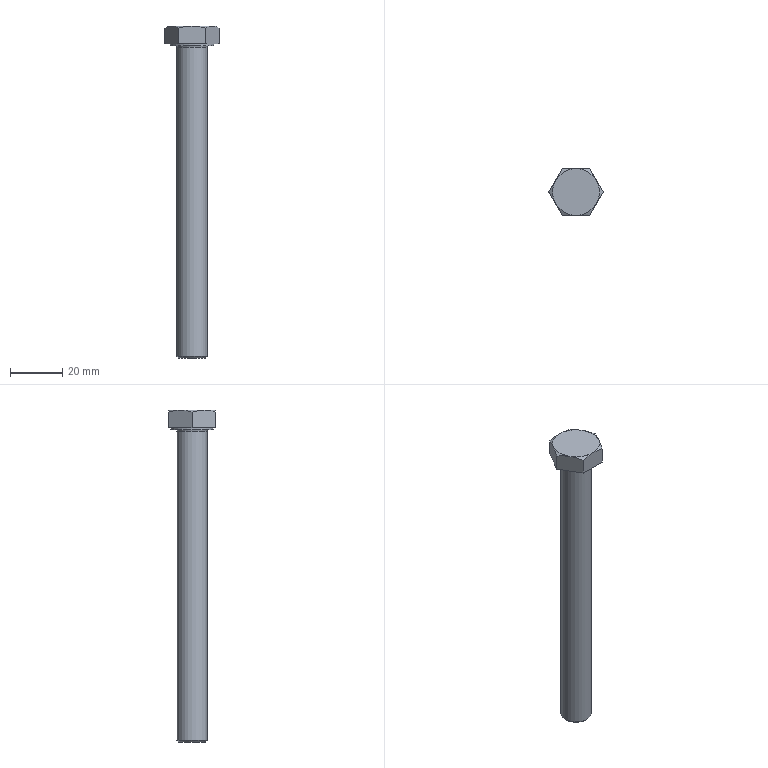Part | NX | features SKETCH 4, EXTRUDE 3, META 3, DATUM_CSYS 2, BLEND 1, CHAMFER 1, LINE 1, SWP104 1, SYMBOLIC_THREAD 1, THREADS 1 | 1 solid | 20 faces | box 20.785 x 18 x 127.5 mm | volume 14961 mm3 | plane 10 | cone 7 | cylinder 2 | torus 1 | commonest cylinder face diameters 11.701 x1 16.63 x1
STEP:
#1=CARTESIAN_POINT('',(5.196,-9.,0.6));
#2=VERTEX_POINT('',#1);
#3=CARTESIAN_POINT('',(10.392,0.,0.6));
#4=VERTEX_POINT('',#3);
#5=CARTESIAN_POINT('',(5.196,-9.,0.6));
#6=DIRECTION('',(0.5,0.866,0.));
#7=VECTOR('',#6,1000.);
#8=LINE('',#5,#7);
#9=EDGE_CURVE('',#2,#4,#8,.T.);
#10=ORIENTED_EDGE('',*,*,#9,.F.);
#11=CARTESIAN_POINT('',(-5.196,-9.,0.6));
#12=VERTEX_POINT('',#11);
#13=CARTESIAN_POINT('',(-5.196,-9.,0.6));
#14=DIRECTION('',(1.,0.,0.));
#15=VECTOR('',#14,1000.);
#16=LINE('',#13,#15);
#17=EDGE_CURVE('',#12,#2,#16,.T.);
#18=ORIENTED_EDGE('',*,*,#17,.F.);
#19=CARTESIAN_POINT('',(-10.392,0.,0.6));
#20=VERTEX_POINT('',#19);
#21=CARTESIAN_POINT('',(-10.392,0.,0.6));
#22=DIRECTION('',(0.5,-0.866,0.));
#23=VECTOR('',#22,1000.);
#24=LINE('',#21,#23);
#25=EDGE_CURVE('',#20,#12,#24,.T.);
#26=ORIENTED_EDGE('',*,*,#25,.F.);
#27=CARTESIAN_POINT('',(-5.196,9.,0.6));
#28=VERTEX_POINT('',#27);
#29=CARTESIAN_POINT('',(-5.196,9.,0.6));
#30=DIRECTION('',(-0.5,-0.866,0.));
#31=VECTOR('',#30,1000.);
#32=LINE('',#29,#31);
#33=EDGE_CURVE('',#28,#20,#32,.T.);
#34=ORIENTED_EDGE('',*,*,#33,.F.);
#35=CARTESIAN_POINT('',(5.196,9.,0.6));
#36=VERTEX_POINT('',#35);
#37=CARTESIAN_POINT('',(5.196,9.,0.6));
#38=DIRECTION('',(-1.,0.,0.));
#39=VECTOR('',#38,1000.);
#40=LINE('',#37,#39);
#41=EDGE_CURVE('',#36,#28,#40,.T.);
#42=ORIENTED_EDGE('',*,*,#41,.F.);
#43=CARTESIAN_POINT('',(10.392,0.,0.6));
#44=DIRECTION('',(-0.5,0.866,0.));
#45=VECTOR('',#44,1000.);
#46=LINE('',#43,#45);
#47=EDGE_CURVE('',#4,#36,#46,.T.);
#48=ORIENTED_EDGE('',*,*,#47,.F.);
#49=EDGE_LOOP('',(#10,#18,#26,#34,#42,#48));
#50=FACE_BOUND('',#49,.T.);
#51=CARTESIAN_POINT('',(8.315,0.,0.6));
#52=VERTEX_POINT('',#51);
#53=CARTESIAN_POINT('',(0.,0.,0.6));
#54=DIRECTION('',(0.,0.,1.));
#55=DIRECTION('',(1.,0.,0.));
#56=AXIS2_PLACEMENT_3D('',#53,#54,#55);
#57=CIRCLE('',#56,8.315);
#58=EDGE_CURVE('',#52,#52,#57,.T.);
#59=ORIENTED_EDGE('',*,*,#58,.T.);
#60=EDGE_LOOP('',(#59));
#61=FACE_BOUND('',#60,.T.);
#62=CARTESIAN_POINT('',(0.,-18.,0.6));
#63=DIRECTION('',(0.,0.,-1.));
#64=DIRECTION('',(-1.,0.,0.));
#65=AXIS2_PLACEMENT_3D('',#62,#63,#64);
#66=PLANE('',#65);
#67=ADVANCED_FACE('',(#50,#61),#66,.T.);
#68=CARTESIAN_POINT('',(5.196,-9.,6.696));
#69=VERTEX_POINT('',#68);
#70=CARTESIAN_POINT('',(7.794,-4.5,7.5));
#71=VERTEX_POINT('',#70);
#72=CARTESIAN_POINT('',(5.196,-9.,6.696));
#73=CARTESIAN_POINT('',(6.046,-7.528,7.187));
#74=CARTESIAN_POINT('',(6.909,-6.033,7.5));
#75=CARTESIAN_POINT('',(7.794,-4.5,7.5));
#76=B_SPLINE_CURVE_WITH_KNOTS('',3,(#72,#73,#74,#75),.UNSPECIFIED.,.F.,.F.,(4,4),(0.000000238,0.005258),.UNSPECIFIED.);
#77=EDGE_CURVE('',#69,#71,#76,.T.);
#78=ORIENTED_EDGE('',*,*,#77,.F.);
#79=CARTESIAN_POINT('',(5.196,-9.,7.5));
#80=DIRECTION('',(0.,0.,-1.));
#81=VECTOR('',#80,1000.);
#82=LINE('',#79,#81);
#83=EDGE_CURVE('',#69,#2,#82,.T.);
#84=ORIENTED_EDGE('',*,*,#83,.T.);
#85=ORIENTED_EDGE('',*,*,#9,.T.);
#86=CARTESIAN_POINT('',(10.392,0.,6.696));
#87=VERTEX_POINT('',#86);
#88=CARTESIAN_POINT('',(10.392,0.,7.5));
#89=DIRECTION('',(0.,0.,-1.));
#90=VECTOR('',#89,1000.);
#91=LINE('',#88,#90);
#92=EDGE_CURVE('',#87,#4,#91,.T.);
#93=ORIENTED_EDGE('',*,*,#92,.F.);
#94=CARTESIAN_POINT('',(7.794,-4.5,7.5));
#95=CARTESIAN_POINT('',(8.676,-2.972,7.5));
#96=CARTESIAN_POINT('',(9.544,-1.469,7.186));
#97=CARTESIAN_POINT('',(10.392,0.,6.696));
#98=B_SPLINE_CURVE_WITH_KNOTS('',3,(#94,#95,#96,#97),.UNSPECIFIED.,.F.,.F.,(4,4),(0.005258,0.0105),.UNSPECIFIED.);
#99=EDGE_CURVE('',#71,#87,#98,.T.);
#100=ORIENTED_EDGE('',*,*,#99,.F.);
#101=EDGE_LOOP('',(#78,#84,#85,#93,#100));
#102=FACE_BOUND('',#101,.T.);
#103=CARTESIAN_POINT('',(5.196,-9.,7.5));
#104=DIRECTION('',(-0.866,0.5,0.));
#105=DIRECTION('',(-0.5,-0.866,0.));
#106=AXIS2_PLACEMENT_3D('',#103,#104,#105);
#107=PLANE('',#106);
#108=ADVANCED_FACE('',(#102),#107,.F.);
#109=CARTESIAN_POINT('',(7.794,4.5,7.5));
#110=VERTEX_POINT('',#109);
#111=CARTESIAN_POINT('',(10.392,0.,6.696));
#112=CARTESIAN_POINT('',(9.542,1.472,7.187));
#113=CARTESIAN_POINT('',(8.679,2.967,7.5));
#114=CARTESIAN_POINT('',(7.794,4.5,7.5));
#115=B_SPLINE_CURVE_WITH_KNOTS('',3,(#111,#112,#113,#114),.UNSPECIFIED.,.F.,.F.,(4,4),(0.000000238,0.005258),.UNSPECIFIED.);
#116=EDGE_CURVE('',#87,#110,#115,.T.);
#117=ORIENTED_EDGE('',*,*,#116,.F.);
#118=ORIENTED_EDGE('',*,*,#92,.T.);
#119=ORIENTED_EDGE('',*,*,#47,.T.);
#120=CARTESIAN_POINT('',(5.196,9.,6.696));
#121=VERTEX_POINT('',#120);
#122=CARTESIAN_POINT('',(5.196,9.,7.5));
#123=DIRECTION('',(0.,0.,-1.));
#124=VECTOR('',#123,1000.);
#125=LINE('',#122,#124);
#126=EDGE_CURVE('',#121,#36,#125,.T.);
#127=ORIENTED_EDGE('',*,*,#126,.F.);
#128=CARTESIAN_POINT('',(7.794,4.5,7.5));
#129=CARTESIAN_POINT('',(6.912,6.028,7.5));
#130=CARTESIAN_POINT('',(6.044,7.531,7.186));
#131=CARTESIAN_POINT('',(5.196,9.,6.696));
#132=B_SPLINE_CURVE_WITH_KNOTS('',3,(#128,#129,#130,#131),.UNSPECIFIED.,.F.,.F.,(4,4),(0.005258,0.0105),.UNSPECIFIED.);
#133=EDGE_CURVE('',#110,#121,#132,.T.);
#134=ORIENTED_EDGE('',*,*,#133,.F.);
#135=EDGE_LOOP('',(#117,#118,#119,#127,#134));
#136=FACE_BOUND('',#135,.T.);
#137=CARTESIAN_POINT('',(10.392,0.,7.5));
#138=DIRECTION('',(-0.866,-0.5,0.));
#139=DIRECTION('',(0.5,-0.866,0.));
#140=AXIS2_PLACEMENT_3D('',#137,#138,#139);
#141=PLANE('',#140);
#142=ADVANCED_FACE('',(#136),#141,.F.);
#143=CARTESIAN_POINT('',(0.,9.,7.5));
#144=VERTEX_POINT('',#143);
#145=CARTESIAN_POINT('',(0.,9.,7.5));
#146=CARTESIAN_POINT('',(1.757,9.,7.5));
#147=CARTESIAN_POINT('',(3.516,9.,7.181));
#148=CARTESIAN_POINT('',(5.196,9.,6.696));
#149=B_SPLINE_CURVE_WITH_KNOTS('',3,(#145,#146,#147,#148),.UNSPECIFIED.,.F.,.F.,(4,4),(0.01453,0.01979),.UNSPECIFIED.);
#150=EDGE_CURVE('',#121,#144,#149,.F.);
#151=ORIENTED_EDGE('',*,*,#150,.F.);
#152=ORIENTED_EDGE('',*,*,#126,.T.);
#153=ORIENTED_EDGE('',*,*,#41,.T.);
#154=CARTESIAN_POINT('',(-5.196,9.,6.696));
#155=VERTEX_POINT('',#154);
#156=CARTESIAN_POINT('',(-5.196,9.,7.5));
#157=DIRECTION('',(0.,0.,-1.));
#158=VECTOR('',#157,1000.);
#159=LINE('',#156,#158);
#160=EDGE_CURVE('',#155,#28,#159,.T.);
#161=ORIENTED_EDGE('',*,*,#160,.F.);
#162=CARTESIAN_POINT('',(-5.196,9.,6.696));
#163=CARTESIAN_POINT('',(-3.506,9.,7.184));
#164=CARTESIAN_POINT('',(-1.756,9.,7.5));
#165=CARTESIAN_POINT('',(0.,9.,7.5));
#166=B_SPLINE_CURVE_WITH_KNOTS('',3,(#162,#163,#164,#165),.UNSPECIFIED.,.F.,.F.,(4,4),(0.009271,0.01453),.UNSPECIFIED.);
#167=EDGE_CURVE('',#144,#155,#166,.F.);
#168=ORIENTED_EDGE('',*,*,#167,.F.);
#169=EDGE_LOOP('',(#151,#152,#153,#161,#168));
#170=FACE_BOUND('',#169,.T.);
#171=CARTESIAN_POINT('',(5.196,9.,7.5));
#172=DIRECTION('',(0.,-1.,0.));
#173=DIRECTION('',(0.,0.,-1.));
#174=AXIS2_PLACEMENT_3D('',#171,#172,#173);
#175=PLANE('',#174);
#176=ADVANCED_FACE('',(#170),#175,.F.);
#177=CARTESIAN_POINT('',(-7.794,4.5,7.5));
#178=VERTEX_POINT('',#177);
#179=CARTESIAN_POINT('',(-5.196,9.,6.696));
#180=CARTESIAN_POINT('',(-6.046,7.528,7.187));
#181=CARTESIAN_POINT('',(-6.909,6.033,7.5));
#182=CARTESIAN_POINT('',(-7.794,4.5,7.5));
#183=B_SPLINE_CURVE_WITH_KNOTS('',3,(#179,#180,#181,#182),.UNSPECIFIED.,.F.,.F.,(4,4),(0.000000238,0.005258),.UNSPECIFIED.);
#184=EDGE_CURVE('',#155,#178,#183,.T.);
#185=ORIENTED_EDGE('',*,*,#184,.F.);
#186=ORIENTED_EDGE('',*,*,#160,.T.);
#187=ORIENTED_EDGE('',*,*,#33,.T.);
#188=CARTESIAN_POINT('',(-10.392,0.,6.696));
#189=VERTEX_POINT('',#188);
#190=CARTESIAN_POINT('',(-10.392,0.,7.5));
#191=DIRECTION('',(0.,0.,-1.));
#192=VECTOR('',#191,1000.);
#193=LINE('',#190,#192);
#194=EDGE_CURVE('',#189,#20,#193,.T.);
#195=ORIENTED_EDGE('',*,*,#194,.F.);
#196=CARTESIAN_POINT('',(-7.794,4.5,7.5));
#197=CARTESIAN_POINT('',(-8.676,2.972,7.5));
#198=CARTESIAN_POINT('',(-9.544,1.469,7.186));
#199=CARTESIAN_POINT('',(-10.392,0.,6.696));
#200=B_SPLINE_CURVE_WITH_KNOTS('',3,(#196,#197,#198,#199),.UNSPECIFIED.,.F.,.F.,(4,4),(0.005258,0.0105),.UNSPECIFIED.);
#201=EDGE_CURVE('',#178,#189,#200,.T.);
#202=ORIENTED_EDGE('',*,*,#201,.F.);
#203=EDGE_LOOP('',(#185,#186,#187,#195,#202));
#204=FACE_BOUND('',#203,.T.);
#205=CARTESIAN_POINT('',(-5.196,9.,7.5));
#206=DIRECTION('',(0.866,-0.5,0.));
#207=DIRECTION('',(0.5,0.866,0.));
#208=AXIS2_PLACEMENT_3D('',#205,#206,#207);
#209=PLANE('',#208);
#210=ADVANCED_FACE('',(#204),#209,.F.);
#211=CARTESIAN_POINT('',(-7.794,-4.5,7.5));
#212=VERTEX_POINT('',#211);
#213=CARTESIAN_POINT('',(-10.392,0.,6.696));
#214=CARTESIAN_POINT('',(-9.542,-1.472,7.187));
#215=CARTESIAN_POINT('',(-8.679,-2.967,7.5));
#216=CARTESIAN_POINT('',(-7.794,-4.5,7.5));
#217=B_SPLINE_CURVE_WITH_KNOTS('',3,(#213,#214,#215,#216),.UNSPECIFIED.,.F.,.F.,(4,4),(0.000000238,0.005258),.UNSPECIFIED.);
#218=EDGE_CURVE('',#189,#212,#217,.T.);
#219=ORIENTED_EDGE('',*,*,#218,.F.);
#220=ORIENTED_EDGE('',*,*,#194,.T.);
#221=ORIENTED_EDGE('',*,*,#25,.T.);
#222=CARTESIAN_POINT('',(-5.196,-9.,6.696));
#223=VERTEX_POINT('',#222);
#224=CARTESIAN_POINT('',(-5.196,-9.,7.5));
#225=DIRECTION('',(0.,0.,-1.));
#226=VECTOR('',#225,1000.);
#227=LINE('',#224,#226);
#228=EDGE_CURVE('',#223,#12,#227,.T.);
#229=ORIENTED_EDGE('',*,*,#228,.F.);
#230=CARTESIAN_POINT('',(-7.794,-4.5,7.5));
#231=CARTESIAN_POINT('',(-6.912,-6.028,7.5));
#232=CARTESIAN_POINT('',(-6.044,-7.531,7.186));
#233=CARTESIAN_POINT('',(-5.196,-9.,6.696));
#234=B_SPLINE_CURVE_WITH_KNOTS('',3,(#230,#231,#232,#233),.UNSPECIFIED.,.F.,.F.,(4,4),(0.005258,0.0105),.UNSPECIFIED.);
#235=EDGE_CURVE('',#212,#223,#234,.T.);
#236=ORIENTED_EDGE('',*,*,#235,.F.);
#237=EDGE_LOOP('',(#219,#220,#221,#229,#236));
#238=FACE_BOUND('',#237,.T.);
#239=CARTESIAN_POINT('',(-10.392,0.,7.5));
#240=DIRECTION('',(0.866,0.5,0.));
#241=DIRECTION('',(-0.5,0.866,0.));
#242=AXIS2_PLACEMENT_3D('',#239,#240,#241);
#243=PLANE('',#242);
#244=ADVANCED_FACE('',(#238),#243,.F.);
#245=CARTESIAN_POINT('',(0.,-9.,7.5));
#246=VERTEX_POINT('',#245);
#247=CARTESIAN_POINT('',(-5.196,-9.,6.696));
#248=CARTESIAN_POINT('',(-3.506,-9.,7.184));
#249=CARTESIAN_POINT('',(-1.756,-9.,7.5));
#250=CARTESIAN_POINT('',(0.,-9.,7.5));
#251=B_SPLINE_CURVE_WITH_KNOTS('',3,(#247,#248,#249,#250),.UNSPECIFIED.,.F.,.F.,(4,4),(0.009271,0.01453),.UNSPECIFIED.);
#252=EDGE_CURVE('',#223,#246,#251,.T.);
#253=ORIENTED_EDGE('',*,*,#252,.F.);
#254=ORIENTED_EDGE('',*,*,#228,.T.);
#255=ORIENTED_EDGE('',*,*,#17,.T.);
#256=ORIENTED_EDGE('',*,*,#83,.F.);
#257=CARTESIAN_POINT('',(0.,-9.,7.5));
#258=CARTESIAN_POINT('',(1.757,-9.,7.5));
#259=CARTESIAN_POINT('',(3.516,-9.,7.181));
#260=CARTESIAN_POINT('',(5.196,-9.,6.696));
#261=B_SPLINE_CURVE_WITH_KNOTS('',3,(#257,#258,#259,#260),.UNSPECIFIED.,.F.,.F.,(4,4),(0.01453,0.01979),.UNSPECIFIED.);
#262=EDGE_CURVE('',#246,#69,#261,.T.);
#263=ORIENTED_EDGE('',*,*,#262,.F.);
#264=EDGE_LOOP('',(#253,#254,#255,#256,#263));
#265=FACE_BOUND('',#264,.T.);
#266=CARTESIAN_POINT('',(-5.196,-9.,7.5));
#267=DIRECTION('',(0.,1.,0.));
#268=DIRECTION('',(0.,0.,1.));
#269=AXIS2_PLACEMENT_3D('',#266,#267,#268);
#270=PLANE('',#269);
#271=ADVANCED_FACE('',(#265),#270,.F.);
#272=ORIENTED_EDGE('',*,*,#77,.T.);
#273=CARTESIAN_POINT('',(0.,0.,7.5));
#274=DIRECTION('',(0.,0.,-1.));
#275=DIRECTION('',(-1.,0.,0.));
#276=AXIS2_PLACEMENT_3D('',#273,#274,#275);
#277=CIRCLE('',#276,9.);
#278=EDGE_CURVE('',#71,#246,#277,.T.);
#279=ORIENTED_EDGE('',*,*,#278,.T.);
#280=ORIENTED_EDGE('',*,*,#262,.T.);
#281=EDGE_LOOP('',(#272,#279,#280));
#282=FACE_BOUND('',#281,.T.);
#283=CARTESIAN_POINT('',(0.,0.,6.696));
#284=DIRECTION('',(0.,0.,-1.));
#285=DIRECTION('',(-1.,0.,0.));
#286=AXIS2_PLACEMENT_3D('',#283,#284,#285);
#287=CONICAL_SURFACE('',#286,10.392,1.047);
#288=ADVANCED_FACE('',(#282),#287,.T.);
#289=ORIENTED_EDGE('',*,*,#235,.T.);
#290=ORIENTED_EDGE('',*,*,#252,.T.);
#291=CARTESIAN_POINT('',(0.,0.,7.5));
#292=DIRECTION('',(0.,0.,-1.));
#293=DIRECTION('',(-1.,0.,0.));
#294=AXIS2_PLACEMENT_3D('',#291,#292,#293);
#295=CIRCLE('',#294,9.);
#296=EDGE_CURVE('',#246,#212,#295,.T.);
#297=ORIENTED_EDGE('',*,*,#296,.T.);
#298=EDGE_LOOP('',(#289,#290,#297));
#299=FACE_BOUND('',#298,.T.);
#300=CARTESIAN_POINT('',(0.,0.,6.696));
#301=DIRECTION('',(0.,0.,-1.));
#302=DIRECTION('',(-1.,0.,0.));
#303=AXIS2_PLACEMENT_3D('',#300,#301,#302);
#304=CONICAL_SURFACE('',#303,10.392,1.047);
#305=ADVANCED_FACE('',(#299),#304,.T.);
#306=ORIENTED_EDGE('',*,*,#201,.T.);
#307=ORIENTED_EDGE('',*,*,#218,.T.);
#308=CARTESIAN_POINT('',(0.,0.,7.5));
#309=DIRECTION('',(0.,0.,-1.));
#310=DIRECTION('',(-1.,0.,0.));
#311=AXIS2_PLACEMENT_3D('',#308,#309,#310);
#312=CIRCLE('',#311,9.);
#313=EDGE_CURVE('',#212,#178,#312,.T.);
#314=ORIENTED_EDGE('',*,*,#313,.T.);
#315=EDGE_LOOP('',(#306,#307,#314));
#316=FACE_BOUND('',#315,.T.);
#317=CARTESIAN_POINT('',(0.,0.,6.696));
#318=DIRECTION('',(0.,0.,-1.));
#319=DIRECTION('',(-1.,0.,0.));
#320=AXIS2_PLACEMENT_3D('',#317,#318,#319);
#321=CONICAL_SURFACE('',#320,10.392,1.047);
#322=ADVANCED_FACE('',(#316),#321,.T.);
#323=ORIENTED_EDGE('',*,*,#167,.T.);
#324=ORIENTED_EDGE('',*,*,#184,.T.);
#325=CARTESIAN_POINT('',(0.,0.,7.5));
#326=DIRECTION('',(0.,0.,-1.));
#327=DIRECTION('',(-1.,0.,0.));
#328=AXIS2_PLACEMENT_3D('',#325,#326,#327);
#329=CIRCLE('',#328,9.);
#330=EDGE_CURVE('',#178,#144,#329,.T.);
#331=ORIENTED_EDGE('',*,*,#330,.T.);
#332=EDGE_LOOP('',(#323,#324,#331));
#333=FACE_BOUND('',#332,.T.);
#334=CARTESIAN_POINT('',(0.,0.,6.696));
#335=DIRECTION('',(0.,0.,-1.));
#336=DIRECTION('',(-1.,0.,0.));
#337=AXIS2_PLACEMENT_3D('',#334,#335,#336);
#338=CONICAL_SURFACE('',#337,10.392,1.047);
#339=ADVANCED_FACE('',(#333),#338,.T.);
#340=ORIENTED_EDGE('',*,*,#133,.T.);
#341=ORIENTED_EDGE('',*,*,#150,.T.);
#342=CARTESIAN_POINT('',(0.,0.,7.5));
#343=DIRECTION('',(0.,0.,-1.));
#344=DIRECTION('',(-1.,0.,0.));
#345=AXIS2_PLACEMENT_3D('',#342,#343,#344);
#346=CIRCLE('',#345,9.);
#347=EDGE_CURVE('',#144,#110,#346,.T.);
#348=ORIENTED_EDGE('',*,*,#347,.T.);
#349=EDGE_LOOP('',(#340,#341,#348));
#350=FACE_BOUND('',#349,.T.);
#351=CARTESIAN_POINT('',(0.,0.,6.696));
#352=DIRECTION('',(0.,0.,-1.));
#353=DIRECTION('',(-1.,0.,0.));
#354=AXIS2_PLACEMENT_3D('',#351,#352,#353);
#355=CONICAL_SURFACE('',#354,10.392,1.047);
#356=ADVANCED_FACE('',(#350),#355,.T.);
#357=ORIENTED_EDGE('',*,*,#99,.T.);
#358=ORIENTED_EDGE('',*,*,#116,.T.);
#359=CARTESIAN_POINT('',(0.,0.,7.5));
#360=DIRECTION('',(0.,0.,-1.));
#361=DIRECTION('',(-1.,0.,0.));
#362=AXIS2_PLACEMENT_3D('',#359,#360,#361);
#363=CIRCLE('',#362,9.);
#364=EDGE_CURVE('',#110,#71,#363,.T.);
#365=ORIENTED_EDGE('',*,*,#364,.T.);
#366=EDGE_LOOP('',(#357,#358,#365));
#367=FACE_BOUND('',#366,.T.);
#368=CARTESIAN_POINT('',(0.,0.,6.696));
#369=DIRECTION('',(0.,0.,-1.));
#370=DIRECTION('',(-1.,0.,0.));
#371=AXIS2_PLACEMENT_3D('',#368,#369,#370);
#372=CONICAL_SURFACE('',#371,10.392,1.047);
#373=ADVANCED_FACE('',(#367),#372,.T.);
#374=ORIENTED_EDGE('',*,*,#330,.F.);
#375=ORIENTED_EDGE('',*,*,#313,.F.);
#376=ORIENTED_EDGE('',*,*,#296,.F.);
#377=ORIENTED_EDGE('',*,*,#278,.F.);
#378=ORIENTED_EDGE('',*,*,#364,.F.);
#379=ORIENTED_EDGE('',*,*,#347,.F.);
#380=EDGE_LOOP('',(#374,#375,#376,#377,#378,#379));
#381=FACE_BOUND('',#380,.T.);
#382=CARTESIAN_POINT('',(0.,-18.,7.5));
#383=DIRECTION('',(0.,0.,-1.));
#384=DIRECTION('',(-1.,0.,0.));
#385=AXIS2_PLACEMENT_3D('',#382,#383,#384);
#386=PLANE('',#385);
#387=ADVANCED_FACE('',(#381),#386,.F.);
#388=ORIENTED_EDGE('',*,*,#58,.F.);
#389=EDGE_LOOP('',(#388));
#390=FACE_BOUND('',#389,.T.);
#391=CARTESIAN_POINT('',(8.315,0.,0.));
#392=VERTEX_POINT('',#391);
#393=CARTESIAN_POINT('',(0.,0.,0.));
#394=DIRECTION('',(0.,0.,1.));
#395=DIRECTION('',(1.,0.,0.));
#396=AXIS2_PLACEMENT_3D('',#393,#394,#395);
#397=CIRCLE('',#396,8.315);
#398=EDGE_CURVE('',#392,#392,#397,.T.);
#399=ORIENTED_EDGE('',*,*,#398,.T.);
#400=EDGE_LOOP('',(#399));
#401=FACE_BOUND('',#400,.T.);
#402=CARTESIAN_POINT('',(0.,0.,0.6));
#403=DIRECTION('',(0.,0.,-1.));
#404=DIRECTION('',(-1.,0.,0.));
#405=AXIS2_PLACEMENT_3D('',#402,#403,#404);
#406=CYLINDRICAL_SURFACE('',#405,8.315);
#407=ADVANCED_FACE('',(#390,#401),#406,.T.);
#408=CARTESIAN_POINT('',(6.45,0.,0.));
#409=VERTEX_POINT('',#408);
#410=CARTESIAN_POINT('',(0.,0.,0.));
#411=DIRECTION('',(0.,0.,1.));
#412=DIRECTION('',(1.,0.,0.));
#413=AXIS2_PLACEMENT_3D('',#410,#411,#412);
#414=CIRCLE('',#413,6.45);
#415=EDGE_CURVE('',#409,#409,#414,.T.);
#416=ORIENTED_EDGE('',*,*,#415,.T.);
#417=EDGE_LOOP('',(#416));
#418=FACE_BOUND('',#417,.T.);
#419=ORIENTED_EDGE('',*,*,#398,.F.);
#420=EDGE_LOOP('',(#419));
#421=FACE_BOUND('',#420,.T.);
#422=CARTESIAN_POINT('',(0.,0.,0.));
#423=DIRECTION('',(0.,0.,1.));
#424=DIRECTION('',(1.,0.,0.));
#425=AXIS2_PLACEMENT_3D('',#422,#423,#424);
#426=PLANE('',#425);
#427=ADVANCED_FACE('',(#418,#421),#426,.F.);
#428=CARTESIAN_POINT('',(5.851,0.,-0.6));
#429=VERTEX_POINT('',#428);
#430=CARTESIAN_POINT('',(0.,0.,-0.6));
#431=DIRECTION('',(0.,0.,1.));
#432=DIRECTION('',(1.,0.,0.));
#433=AXIS2_PLACEMENT_3D('',#430,#431,#432);
#434=CIRCLE('',#433,5.851);
#435=EDGE_CURVE('',#429,#429,#434,.F.);
#436=ORIENTED_EDGE('',*,*,#435,.T.);
#437=EDGE_LOOP('',(#436));
#438=FACE_BOUND('',#437,.T.);
#439=CARTESIAN_POINT('',(5.851,0.,-119.415));
#440=VERTEX_POINT('',#439);
#441=CARTESIAN_POINT('',(0.,0.,-119.415));
#442=DIRECTION('',(0.,0.,1.));
#443=DIRECTION('',(1.,0.,0.));
#444=AXIS2_PLACEMENT_3D('',#441,#442,#443);
#445=CIRCLE('',#444,5.851);
#446=EDGE_CURVE('',#440,#440,#445,.T.);
#447=ORIENTED_EDGE('',*,*,#446,.T.);
#448=EDGE_LOOP('',(#447));
#449=FACE_BOUND('',#448,.T.);
#450=CARTESIAN_POINT('',(0.,0.,-120.));
#451=DIRECTION('',(0.,0.,1.));
#452=DIRECTION('',(1.,0.,0.));
#453=AXIS2_PLACEMENT_3D('',#450,#451,#452);
#454=CYLINDRICAL_SURFACE('',#453,5.851);
#455=ADVANCED_FACE('',(#438,#449),#454,.T.);
#456=CARTESIAN_POINT('',(5.265,0.,-120.));
#457=VERTEX_POINT('',#456);
#458=CARTESIAN_POINT('',(0.,0.,-120.));
#459=DIRECTION('',(0.,0.,1.));
#460=DIRECTION('',(1.,0.,0.));
#461=AXIS2_PLACEMENT_3D('',#458,#459,#460);
#462=CIRCLE('',#461,5.265);
#463=EDGE_CURVE('',#457,#457,#462,.F.);
#464=ORIENTED_EDGE('',*,*,#463,.T.);
#465=EDGE_LOOP('',(#464));
#466=FACE_BOUND('',#465,.T.);
#467=CARTESIAN_POINT('',(0.,0.,-120.));
#468=DIRECTION('',(0.,0.,1.));
#469=DIRECTION('',(1.,0.,0.));
#470=AXIS2_PLACEMENT_3D('',#467,#468,#469);
#471=PLANE('',#470);
#472=ADVANCED_FACE('',(#466),#471,.F.);
#473=ORIENTED_EDGE('',*,*,#463,.F.);
#474=EDGE_LOOP('',(#473));
#475=FACE_BOUND('',#474,.T.);
#476=ORIENTED_EDGE('',*,*,#446,.F.);
#477=EDGE_LOOP('',(#476));
#478=FACE_BOUND('',#477,.T.);
#479=CARTESIAN_POINT('',(0.,0.,-119.415));
#480=DIRECTION('',(0.,0.,1.));
#481=DIRECTION('',(1.,0.,0.));
#482=AXIS2_PLACEMENT_3D('',#479,#480,#481);
#483=CONICAL_SURFACE('',#482,5.851,0.7854);
#484=ADVANCED_FACE('',(#475,#478),#483,.T.);
#485=ORIENTED_EDGE('',*,*,#435,.F.);
#486=EDGE_LOOP('',(#485));
#487=FACE_BOUND('',#486,.T.);
#488=ORIENTED_EDGE('',*,*,#415,.F.);
#489=EDGE_LOOP('',(#488));
#490=FACE_BOUND('',#489,.T.);
#491=CARTESIAN_POINT('',(0.,0.,-0.6));
#492=DIRECTION('',(0.,0.,1.));
#493=DIRECTION('',(1.,0.,0.));
#494=AXIS2_PLACEMENT_3D('',#491,#492,#493);
#495=TOROIDAL_SURFACE('',#494,6.45,0.6);
#496=ADVANCED_FACE('',(#487,#490),#495,.F.);
#497=CLOSED_SHELL('',(#67,#108,#142,#176,#210,#244,#271,#288,#305,#322,#339,#356,#373,#387,#407,#427,#455,#472,#484,#496));
#498=MANIFOLD_SOLID_BREP('',#497);
#499=(LENGTH_UNIT()NAMED_UNIT(*)SI_UNIT(.MILLI.,.METRE.));
#500=UNCERTAINTY_MEASURE_WITH_UNIT(LENGTH_MEASURE(0.0508),#499,'','');
#501=(NAMED_UNIT(*)PLANE_ANGLE_UNIT()SI_UNIT($,.RADIAN.));
#502=(NAMED_UNIT(*)SI_UNIT($,.STERADIAN.)SOLID_ANGLE_UNIT());
#503=(GEOMETRIC_REPRESENTATION_CONTEXT(3)GLOBAL_UNCERTAINTY_ASSIGNED_CONTEXT((#500))GLOBAL_UNIT_ASSIGNED_CONTEXT((#499,#501,#502))REPRESENTATION_CONTEXT('',''));
#504=ADVANCED_BREP_SHAPE_REPRESENTATION('',(#498),#503);